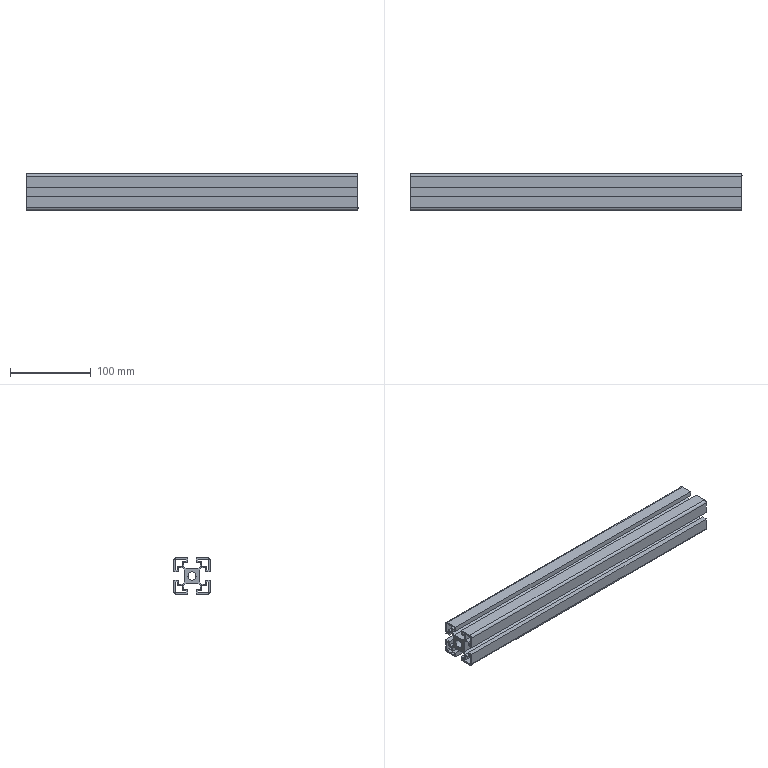Part | STEP file | bosch_3842990520_4g1k76bwvav0hbf1r78r1itfr | 1 solid | 87 faces | box 410 x 45 x 45 mm | volume 335275 mm3 | plane 78 | cylinder 9 | commonest cylinder face diameters 2 x4 6 x4 10 x1